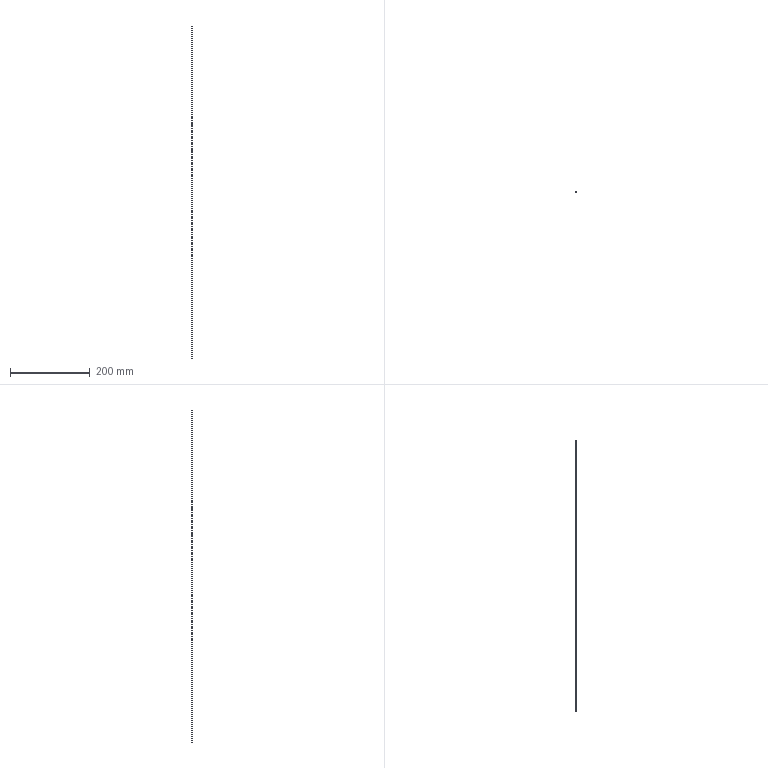Part | STEP file | PZ-G51EP-Part-1-10 | 1 solid | 4 faces | box 1 x 1 x 833 mm | volume 654.237 mm3 | cylinder 2 | plane 2 | commonest cylinder face diameters 1 x2
STEP:
#1=CARTESIAN_POINT('',(-0.5,4.,823.));
#2=VERTEX_POINT('',#1);
#3=CARTESIAN_POINT('',(0.5,4.,823.));
#4=VERTEX_POINT('',#3);
#5=CARTESIAN_POINT('',(0.,4.,823.));
#6=DIRECTION('',(0.,0.,-1.));
#7=DIRECTION('',(-1.,0.,0.));
#8=AXIS2_PLACEMENT_3D('',#5,#6,#7);
#9=CIRCLE('',#8,0.5);
#10=EDGE_CURVE('',#2,#4,#9,.T.);
#11=ORIENTED_EDGE('',*,*,#10,.T.);
#12=CARTESIAN_POINT('',(0.5,4.,-10.));
#13=VERTEX_POINT('',#12);
#14=CARTESIAN_POINT('',(0.5,4.,823.));
#15=DIRECTION('',(0.,0.,-1.));
#16=VECTOR('',#15,1000.);
#17=LINE('',#14,#16);
#18=EDGE_CURVE('',#4,#13,#17,.T.);
#19=ORIENTED_EDGE('',*,*,#18,.T.);
#20=CARTESIAN_POINT('',(-0.5,4.,-10.));
#21=VERTEX_POINT('',#20);
#22=CARTESIAN_POINT('',(0.,4.,-10.));
#23=DIRECTION('',(0.,0.,1.));
#24=DIRECTION('',(1.,0.,0.));
#25=AXIS2_PLACEMENT_3D('',#22,#23,#24);
#26=CIRCLE('',#25,0.5);
#27=EDGE_CURVE('',#13,#21,#26,.T.);
#28=ORIENTED_EDGE('',*,*,#27,.T.);
#29=CARTESIAN_POINT('',(-0.5,4.,823.));
#30=DIRECTION('',(0.,0.,-1.));
#31=VECTOR('',#30,1000.);
#32=LINE('',#29,#31);
#33=EDGE_CURVE('',#2,#21,#32,.T.);
#34=ORIENTED_EDGE('',*,*,#33,.F.);
#35=EDGE_LOOP('',(#11,#19,#28,#34));
#36=FACE_OUTER_BOUND('',#35,.T.);
#37=CARTESIAN_POINT('',(0.,4.,823.));
#38=DIRECTION('',(0.,0.,-1.));
#39=DIRECTION('',(-1.,0.,0.));
#40=AXIS2_PLACEMENT_3D('',#37,#38,#39);
#41=CYLINDRICAL_SURFACE('',#40,0.5);
#42=ADVANCED_FACE('',(#36),#41,.T.);
#43=CARTESIAN_POINT('',(0.,4.,-10.));
#44=DIRECTION('',(0.,0.,1.));
#45=DIRECTION('',(1.,0.,0.));
#46=AXIS2_PLACEMENT_3D('',#43,#44,#45);
#47=CIRCLE('',#46,0.5);
#48=EDGE_CURVE('',#21,#13,#47,.T.);
#49=ORIENTED_EDGE('',*,*,#48,.F.);
#50=ORIENTED_EDGE('',*,*,#27,.F.);
#51=EDGE_LOOP('',(#49,#50));
#52=FACE_OUTER_BOUND('',#51,.T.);
#53=CARTESIAN_POINT('',(0.,4.,-10.));
#54=DIRECTION('',(0.,0.,-1.));
#55=DIRECTION('',(-1.,0.,0.));
#56=AXIS2_PLACEMENT_3D('',#53,#54,#55);
#57=PLANE('',#56);
#58=ADVANCED_FACE('',(#52),#57,.T.);
#59=ORIENTED_EDGE('',*,*,#10,.F.);
#60=CARTESIAN_POINT('',(0.,4.,823.));
#61=DIRECTION('',(0.,0.,-1.));
#62=DIRECTION('',(-1.,0.,0.));
#63=AXIS2_PLACEMENT_3D('',#60,#61,#62);
#64=CIRCLE('',#63,0.5);
#65=EDGE_CURVE('',#4,#2,#64,.T.);
#66=ORIENTED_EDGE('',*,*,#65,.F.);
#67=EDGE_LOOP('',(#59,#66));
#68=FACE_OUTER_BOUND('',#67,.T.);
#69=CARTESIAN_POINT('',(0.,4.,823.));
#70=DIRECTION('',(0.,0.,1.));
#71=DIRECTION('',(1.,0.,0.));
#72=AXIS2_PLACEMENT_3D('',#69,#70,#71);
#73=PLANE('',#72);
#74=ADVANCED_FACE('',(#68),#73,.T.);
#75=ORIENTED_EDGE('',*,*,#18,.F.);
#76=ORIENTED_EDGE('',*,*,#65,.T.);
#77=ORIENTED_EDGE('',*,*,#33,.T.);
#78=ORIENTED_EDGE('',*,*,#48,.T.);
#79=EDGE_LOOP('',(#75,#76,#77,#78));
#80=FACE_OUTER_BOUND('',#79,.T.);
#81=CARTESIAN_POINT('',(0.,4.,823.));
#82=DIRECTION('',(0.,0.,-1.));
#83=DIRECTION('',(-1.,0.,0.));
#84=AXIS2_PLACEMENT_3D('',#81,#82,#83);
#85=CYLINDRICAL_SURFACE('',#84,0.5);
#86=ADVANCED_FACE('',(#80),#85,.T.);
#87=CLOSED_SHELL('',(#42,#58,#74,#86));
#88=MANIFOLD_SOLID_BREP('',#87);
#89=CARTESIAN_POINT('',(0.,0.,0.));
#90=DIRECTION('',(0.,0.,1.));
#91=DIRECTION('',(1.,0.,0.));
#92=AXIS2_PLACEMENT_3D('',#89,#90,#91);
#93=(LENGTH_UNIT()NAMED_UNIT(*)SI_UNIT(.MILLI.,.METRE.));
#94=UNCERTAINTY_MEASURE_WITH_UNIT(LENGTH_MEASURE(0.00001),#93,'','');
#95=(NAMED_UNIT(*)PLANE_ANGLE_UNIT()SI_UNIT($,.RADIAN.));
#96=(NAMED_UNIT(*)SI_UNIT($,.STERADIAN.)SOLID_ANGLE_UNIT());
#97=(GEOMETRIC_REPRESENTATION_CONTEXT(3)GLOBAL_UNCERTAINTY_ASSIGNED_CONTEXT((#94))GLOBAL_UNIT_ASSIGNED_CONTEXT((#93,#95,#96))REPRESENTATION_CONTEXT('',''));
#98=ADVANCED_BREP_SHAPE_REPRESENTATION('',(#88,#92),#97);